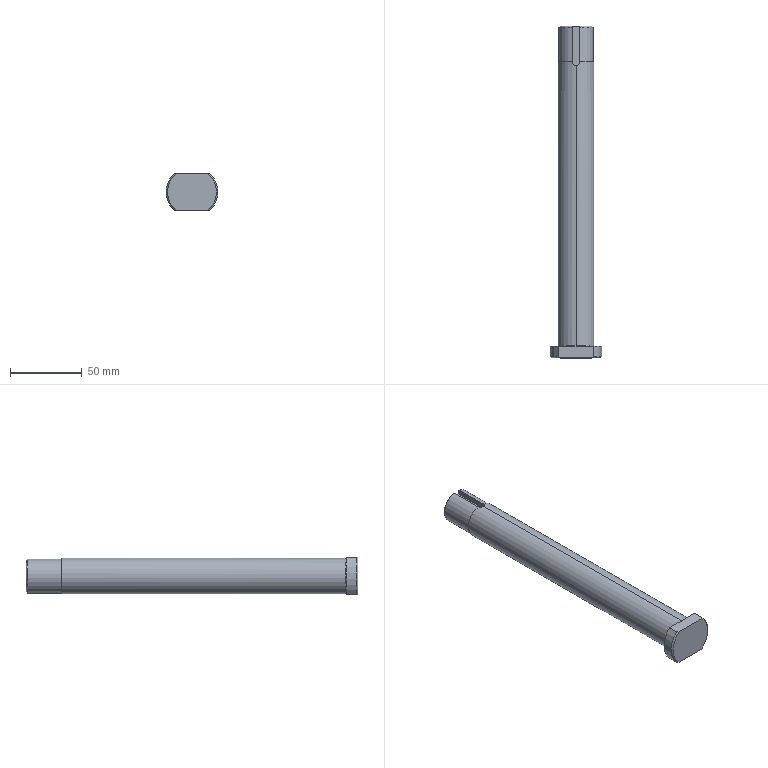Part | SolidWorks | features Chamfer 2, Fillet 2, ICE 2, Revolution 1 | 1 solid | 22 faces | box 36 x 231 x 26 mm | volume 114684 mm3 | plane 10 | cylinder 6 | cone 4 | torus 2 | commonest cylinder face diameters 25 x2 36 x2 5 x1 24 x1
STEP:
#1=CARTESIAN_POINT('',(0.,8.,13.));
#2=VERTEX_POINT('',#1);
#3=CARTESIAN_POINT('',(0.,8.,-13.));
#4=VERTEX_POINT('',#3);
#5=CARTESIAN_POINT('',(0.,8.,0.));
#6=DIRECTION('',(0.,-1.,0.));
#7=DIRECTION('',(0.,0.,-1.));
#8=AXIS2_PLACEMENT_3D('',#5,#6,#7);
#9=CIRCLE('',#8,13.);
#10=EDGE_CURVE('',#2,#4,#9,.T.);
#11=ORIENTED_EDGE('',*,*,#10,.F.);
#12=CARTESIAN_POINT('',(0.,8.5,12.5));
#13=VERTEX_POINT('',#12);
#14=CARTESIAN_POINT('',(0.,8.5,13.));
#15=DIRECTION('',(1.,0.,0.));
#16=DIRECTION('',(0.,0.,-1.));
#17=AXIS2_PLACEMENT_3D('',#14,#15,#16);
#18=CIRCLE('',#17,0.5);
#19=EDGE_CURVE('',#2,#13,#18,.T.);
#20=ORIENTED_EDGE('',*,*,#19,.T.);
#21=CARTESIAN_POINT('',(0.,8.5,-12.5));
#22=VERTEX_POINT('',#21);
#23=CARTESIAN_POINT('',(0.,8.5,0.));
#24=DIRECTION('',(0.,1.,0.));
#25=DIRECTION('',(0.,0.,-1.));
#26=AXIS2_PLACEMENT_3D('',#23,#24,#25);
#27=CIRCLE('',#26,12.5);
#28=EDGE_CURVE('',#22,#13,#27,.T.);
#29=ORIENTED_EDGE('',*,*,#28,.F.);
#30=CARTESIAN_POINT('',(0.,8.5,-13.));
#31=DIRECTION('',(-1.,0.,0.));
#32=DIRECTION('',(0.,0.,1.));
#33=AXIS2_PLACEMENT_3D('',#30,#31,#32);
#34=CIRCLE('',#33,0.5);
#35=EDGE_CURVE('',#4,#22,#34,.T.);
#36=ORIENTED_EDGE('',*,*,#35,.F.);
#37=EDGE_LOOP('',(#11,#20,#29,#36));
#38=FACE_OUTER_BOUND('',#37,.T.);
#39=CARTESIAN_POINT('',(0.,8.5,0.));
#40=DIRECTION('',(0.,-1.,0.));
#41=DIRECTION('',(0.,0.,-1.));
#42=AXIS2_PLACEMENT_3D('',#39,#40,#41);
#43=TOROIDAL_SURFACE('',#42,13.,0.5);
#44=ADVANCED_FACE('',(#38),#43,.F.);
#45=CARTESIAN_POINT('',(0.,231.,-11.));
#46=VERTEX_POINT('',#45);
#47=CARTESIAN_POINT('',(-2.5,231.,10.712));
#48=VERTEX_POINT('',#47);
#49=CARTESIAN_POINT('',(0.,231.,0.));
#50=DIRECTION('',(0.,1.,0.));
#51=DIRECTION('',(0.,0.,-1.));
#52=AXIS2_PLACEMENT_3D('',#49,#50,#51);
#53=CIRCLE('',#52,11.);
#54=EDGE_CURVE('',#46,#48,#53,.T.);
#55=ORIENTED_EDGE('',*,*,#54,.F.);
#56=CARTESIAN_POINT('',(0.,230.,-12.));
#57=VERTEX_POINT('',#56);
#58=CARTESIAN_POINT('',(0.,231.,-11.));
#59=DIRECTION('',(0.,-0.7071,-0.7071));
#60=VECTOR('',#59,1000.);
#61=LINE('',#58,#60);
#62=EDGE_CURVE('',#46,#57,#61,.T.);
#63=ORIENTED_EDGE('',*,*,#62,.T.);
#64=CARTESIAN_POINT('',(-2.5,230.,11.737));
#65=VERTEX_POINT('',#64);
#66=CARTESIAN_POINT('',(0.,230.,0.));
#67=DIRECTION('',(0.,-1.,0.));
#68=DIRECTION('',(0.,0.,-1.));
#69=AXIS2_PLACEMENT_3D('',#66,#67,#68);
#70=CIRCLE('',#69,12.);
#71=EDGE_CURVE('',#65,#57,#70,.T.);
#72=ORIENTED_EDGE('',*,*,#71,.F.);
#73=CARTESIAN_POINT('',(-2.5,231.,10.712));
#74=CARTESIAN_POINT('',(-2.5,230.667,11.054));
#75=CARTESIAN_POINT('',(-2.5,230.334,11.396));
#76=CARTESIAN_POINT('',(-2.5,230.,11.737));
#77=B_SPLINE_CURVE_WITH_KNOTS('',3,(#73,#74,#75,#76),.UNSPECIFIED.,.F.,.F.,(4,4),(0.,0.001432),.UNSPECIFIED.);
#78=EDGE_CURVE('',#48,#65,#77,.T.);
#79=ORIENTED_EDGE('',*,*,#78,.F.);
#80=EDGE_LOOP('',(#55,#63,#72,#79));
#81=FACE_OUTER_BOUND('',#80,.T.);
#82=CARTESIAN_POINT('',(0.,231.,0.));
#83=DIRECTION('',(0.,-1.,0.));
#84=DIRECTION('',(0.,0.,-1.));
#85=AXIS2_PLACEMENT_3D('',#82,#83,#84);
#86=CONICAL_SURFACE('',#85,11.,0.7854);
#87=ADVANCED_FACE('',(#81),#86,.T.);
#88=CARTESIAN_POINT('',(0.,8.5,0.));
#89=DIRECTION('',(0.,1.,0.));
#90=DIRECTION('',(0.,0.,-1.));
#91=AXIS2_PLACEMENT_3D('',#88,#89,#90);
#92=CIRCLE('',#91,12.5);
#93=EDGE_CURVE('',#13,#22,#92,.T.);
#94=ORIENTED_EDGE('',*,*,#93,.T.);
#95=CARTESIAN_POINT('',(0.,206.,-12.5));
#96=VERTEX_POINT('',#95);
#97=CARTESIAN_POINT('',(0.,0.,-12.5));
#98=DIRECTION('',(0.,1.,0.));
#99=VECTOR('',#98,1000.);
#100=LINE('',#97,#99);
#101=EDGE_CURVE('',#22,#96,#100,.T.);
#102=ORIENTED_EDGE('',*,*,#101,.T.);
#103=CARTESIAN_POINT('',(2.5,206.,12.247));
#104=VERTEX_POINT('',#103);
#105=CARTESIAN_POINT('',(0.,206.,0.));
#106=DIRECTION('',(0.,1.,0.));
#107=DIRECTION('',(0.,0.,1.));
#108=AXIS2_PLACEMENT_3D('',#105,#106,#107);
#109=CIRCLE('',#108,12.5);
#110=EDGE_CURVE('',#104,#96,#109,.T.);
#111=ORIENTED_EDGE('',*,*,#110,.F.);
#112=CARTESIAN_POINT('',(0.,203.5,12.5));
#113=VERTEX_POINT('',#112);
#114=CARTESIAN_POINT('',(2.5,206.,12.247));
#115=CARTESIAN_POINT('',(2.5,205.834,12.247));
#116=CARTESIAN_POINT('',(2.484,205.672,12.251));
#117=CARTESIAN_POINT('',(2.42,205.351,12.264));
#118=CARTESIAN_POINT('',(2.372,205.192,12.273));
#119=CARTESIAN_POINT('',(2.246,204.89,12.297));
#120=CARTESIAN_POINT('',(2.169,204.746,12.311));
#121=CARTESIAN_POINT('',(1.987,204.475,12.341));
#122=CARTESIAN_POINT('',(1.882,204.346,12.358));
#123=CARTESIAN_POINT('',(1.537,204.002,12.407));
#124=CARTESIAN_POINT('',(1.258,203.815,12.44));
#125=CARTESIAN_POINT('',(0.8073,203.628,12.475));
#126=CARTESIAN_POINT('',(0.6491,203.58,12.484));
#127=CARTESIAN_POINT('',(0.3261,203.516,12.497));
#128=CARTESIAN_POINT('',(0.1636,203.5,12.5));
#129=CARTESIAN_POINT('',(0.,203.5,12.5));
#130=B_SPLINE_CURVE_WITH_KNOTS('',3,(#114,#115,#116,#117,#118,#119,#120,#121,#122,#123,#124,#125,#126,#127,#128,#129),.UNSPECIFIED.,.F.,.F.,(4,2,2,2,2,2,2,4),(0.,0.0004899,0.0009797,0.00147,0.001959,0.002939,0.003429,0.003919),.UNSPECIFIED.);
#131=EDGE_CURVE('',#104,#113,#130,.T.);
#132=ORIENTED_EDGE('',*,*,#131,.T.);
#133=CARTESIAN_POINT('',(0.,0.,12.5));
#134=DIRECTION('',(0.,1.,0.));
#135=VECTOR('',#134,1000.);
#136=LINE('',#133,#135);
#137=EDGE_CURVE('',#13,#113,#136,.T.);
#138=ORIENTED_EDGE('',*,*,#137,.F.);
#139=EDGE_LOOP('',(#94,#102,#111,#132,#138));
#140=FACE_OUTER_BOUND('',#139,.T.);
#141=CARTESIAN_POINT('',(0.,0.,0.));
#142=DIRECTION('',(0.,1.,0.));
#143=DIRECTION('',(0.,0.,1.));
#144=AXIS2_PLACEMENT_3D('',#141,#142,#143);
#145=CYLINDRICAL_SURFACE('',#144,12.5);
#146=ADVANCED_FACE('',(#140),#145,.T.);
#147=CARTESIAN_POINT('',(-12.45,8.,13.));
#148=VERTEX_POINT('',#147);
#149=CARTESIAN_POINT('',(18.,8.,13.));
#150=DIRECTION('',(1.,0.,0.));
#151=VECTOR('',#150,1000.);
#152=LINE('',#149,#151);
#153=EDGE_CURVE('',#148,#2,#152,.T.);
#154=ORIENTED_EDGE('',*,*,#153,.T.);
#155=ORIENTED_EDGE('',*,*,#10,.T.);
#156=CARTESIAN_POINT('',(-12.45,8.,-13.));
#157=VERTEX_POINT('',#156);
#158=CARTESIAN_POINT('',(18.,8.,-13.));
#159=DIRECTION('',(-1.,0.,0.));
#160=VECTOR('',#159,1000.);
#161=LINE('',#158,#160);
#162=EDGE_CURVE('',#4,#157,#161,.T.);
#163=ORIENTED_EDGE('',*,*,#162,.T.);
#164=CARTESIAN_POINT('',(0.,8.,0.));
#165=DIRECTION('',(0.,1.,0.));
#166=DIRECTION('',(0.,0.,1.));
#167=AXIS2_PLACEMENT_3D('',#164,#165,#166);
#168=CIRCLE('',#167,18.);
#169=EDGE_CURVE('',#157,#148,#168,.T.);
#170=ORIENTED_EDGE('',*,*,#169,.T.);
#171=EDGE_LOOP('',(#154,#155,#163,#170));
#172=FACE_OUTER_BOUND('',#171,.T.);
#173=CARTESIAN_POINT('',(18.,8.,0.));
#174=DIRECTION('',(0.,-1.,0.));
#175=DIRECTION('',(0.,0.,-1.));
#176=AXIS2_PLACEMENT_3D('',#173,#174,#175);
#177=PLANE('',#176);
#178=ADVANCED_FACE('',(#172),#177,.F.);
#179=ORIENTED_EDGE('',*,*,#101,.F.);
#180=ORIENTED_EDGE('',*,*,#28,.T.);
#181=ORIENTED_EDGE('',*,*,#137,.T.);
#182=CARTESIAN_POINT('',(-2.5,206.,12.247));
#183=VERTEX_POINT('',#182);
#184=CARTESIAN_POINT('',(0.,203.5,12.5));
#185=CARTESIAN_POINT('',(-0.1634,203.5,12.5));
#186=CARTESIAN_POINT('',(-0.3294,203.516,12.497));
#187=CARTESIAN_POINT('',(-0.6501,203.58,12.484));
#188=CARTESIAN_POINT('',(-0.806,203.628,12.475));
#189=CARTESIAN_POINT('',(-1.109,203.753,12.452));
#190=CARTESIAN_POINT('',(-1.255,203.832,12.438));
#191=CARTESIAN_POINT('',(-1.525,204.012,12.407));
#192=CARTESIAN_POINT('',(-1.651,204.116,12.391));
#193=CARTESIAN_POINT('',(-1.884,204.348,12.358));
#194=CARTESIAN_POINT('',(-1.987,204.474,12.341));
#195=CARTESIAN_POINT('',(-2.168,204.744,12.311));
#196=CARTESIAN_POINT('',(-2.246,204.89,12.297));
#197=CARTESIAN_POINT('',(-2.371,205.192,12.273));
#198=CARTESIAN_POINT('',(-2.419,205.348,12.264));
#199=CARTESIAN_POINT('',(-2.483,205.669,12.251));
#200=CARTESIAN_POINT('',(-2.5,205.834,12.247));
#201=CARTESIAN_POINT('',(-2.5,206.,12.247));
#202=B_SPLINE_CURVE_WITH_KNOTS('',3,(#184,#185,#186,#187,#188,#189,#190,#191,#192,#193,#194,#195,#196,#197,#198,#199,#200,#201),.UNSPECIFIED.,.F.,.F.,(4,2,2,2,2,2,2,2,4),(0.003919,0.004408,0.004898,0.005387,0.005876,0.006366,0.006855,0.007344,0.007834),.UNSPECIFIED.);
#203=EDGE_CURVE('',#113,#183,#202,.T.);
#204=ORIENTED_EDGE('',*,*,#203,.T.);
#205=CARTESIAN_POINT('',(0.,206.,0.));
#206=DIRECTION('',(0.,1.,0.));
#207=DIRECTION('',(0.,0.,1.));
#208=AXIS2_PLACEMENT_3D('',#205,#206,#207);
#209=CIRCLE('',#208,12.5);
#210=EDGE_CURVE('',#96,#183,#209,.T.);
#211=ORIENTED_EDGE('',*,*,#210,.F.);
#212=EDGE_LOOP('',(#179,#180,#181,#204,#211));
#213=FACE_OUTER_BOUND('',#212,.T.);
#214=CARTESIAN_POINT('',(0.,0.,0.));
#215=DIRECTION('',(0.,1.,0.));
#216=DIRECTION('',(0.,0.,1.));
#217=AXIS2_PLACEMENT_3D('',#214,#215,#216);
#218=CYLINDRICAL_SURFACE('',#217,12.5);
#219=ADVANCED_FACE('',(#213),#218,.T.);
#220=CARTESIAN_POINT('',(-2.5,206.,11.737));
#221=VERTEX_POINT('',#220);
#222=CARTESIAN_POINT('',(-2.5,206.,13.001));
#223=DIRECTION('',(0.,0.,-1.));
#224=VECTOR('',#223,1000.);
#225=LINE('',#222,#224);
#226=EDGE_CURVE('',#183,#221,#225,.T.);
#227=ORIENTED_EDGE('',*,*,#226,.T.);
#228=CARTESIAN_POINT('',(2.5,206.,11.737));
#229=VERTEX_POINT('',#228);
#230=CARTESIAN_POINT('',(0.,206.,0.));
#231=DIRECTION('',(0.,1.,0.));
#232=DIRECTION('',(0.,0.,1.));
#233=AXIS2_PLACEMENT_3D('',#230,#231,#232);
#234=CIRCLE('',#233,12.);
#235=EDGE_CURVE('',#229,#221,#234,.T.);
#236=ORIENTED_EDGE('',*,*,#235,.F.);
#237=CARTESIAN_POINT('',(2.5,206.,13.001));
#238=DIRECTION('',(0.,0.,-1.));
#239=VECTOR('',#238,1000.);
#240=LINE('',#237,#239);
#241=EDGE_CURVE('',#104,#229,#240,.T.);
#242=ORIENTED_EDGE('',*,*,#241,.F.);
#243=ORIENTED_EDGE('',*,*,#110,.T.);
#244=ORIENTED_EDGE('',*,*,#210,.T.);
#245=EDGE_LOOP('',(#227,#236,#242,#243,#244));
#246=FACE_OUTER_BOUND('',#245,.T.);
#247=CARTESIAN_POINT('',(12.5,206.,0.));
#248=DIRECTION('',(0.,-1.,0.));
#249=DIRECTION('',(0.,0.,-1.));
#250=AXIS2_PLACEMENT_3D('',#247,#248,#249);
#251=PLANE('',#250);
#252=ADVANCED_FACE('',(#246),#251,.F.);
#253=CARTESIAN_POINT('',(-2.5,0.,11.737));
#254=DIRECTION('',(0.,1.,0.));
#255=VECTOR('',#254,1000.);
#256=LINE('',#253,#255);
#257=EDGE_CURVE('',#221,#65,#256,.T.);
#258=ORIENTED_EDGE('',*,*,#257,.T.);
#259=ORIENTED_EDGE('',*,*,#71,.T.);
#260=CARTESIAN_POINT('',(2.5,230.,11.737));
#261=VERTEX_POINT('',#260);
#262=CARTESIAN_POINT('',(0.,230.,0.));
#263=DIRECTION('',(0.,-1.,0.));
#264=DIRECTION('',(0.,0.,-1.));
#265=AXIS2_PLACEMENT_3D('',#262,#263,#264);
#266=CIRCLE('',#265,12.);
#267=EDGE_CURVE('',#57,#261,#266,.T.);
#268=ORIENTED_EDGE('',*,*,#267,.T.);
#269=CARTESIAN_POINT('',(2.5,0.,11.737));
#270=DIRECTION('',(0.,-1.,0.));
#271=VECTOR('',#270,1000.);
#272=LINE('',#269,#271);
#273=EDGE_CURVE('',#261,#229,#272,.T.);
#274=ORIENTED_EDGE('',*,*,#273,.T.);
#275=ORIENTED_EDGE('',*,*,#235,.T.);
#276=EDGE_LOOP('',(#258,#259,#268,#274,#275));
#277=FACE_OUTER_BOUND('',#276,.T.);
#278=CARTESIAN_POINT('',(0.,0.,0.));
#279=DIRECTION('',(0.,1.,0.));
#280=DIRECTION('',(0.,0.,1.));
#281=AXIS2_PLACEMENT_3D('',#278,#279,#280);
#282=CYLINDRICAL_SURFACE('',#281,12.);
#283=ADVANCED_FACE('',(#277),#282,.T.);
#284=CARTESIAN_POINT('',(2.5,231.,8.));
#285=VERTEX_POINT('',#284);
#286=CARTESIAN_POINT('',(2.5,231.,10.712));
#287=VERTEX_POINT('',#286);
#288=CARTESIAN_POINT('',(2.5,231.,13.001));
#289=DIRECTION('',(0.,0.,1.));
#290=VECTOR('',#289,1000.);
#291=LINE('',#288,#290);
#292=EDGE_CURVE('',#285,#287,#291,.T.);
#293=ORIENTED_EDGE('',*,*,#292,.T.);
#294=CARTESIAN_POINT('',(0.,231.,0.));
#295=DIRECTION('',(0.,1.,0.));
#296=DIRECTION('',(0.,0.,-1.));
#297=AXIS2_PLACEMENT_3D('',#294,#295,#296);
#298=CIRCLE('',#297,11.);
#299=EDGE_CURVE('',#287,#46,#298,.T.);
#300=ORIENTED_EDGE('',*,*,#299,.T.);
#301=ORIENTED_EDGE('',*,*,#54,.T.);
#302=CARTESIAN_POINT('',(-2.5,231.,8.));
#303=VERTEX_POINT('',#302);
#304=CARTESIAN_POINT('',(-2.5,231.,13.001));
#305=DIRECTION('',(0.,0.,-1.));
#306=VECTOR('',#305,1000.);
#307=LINE('',#304,#306);
#308=EDGE_CURVE('',#48,#303,#307,.T.);
#309=ORIENTED_EDGE('',*,*,#308,.T.);
#310=CARTESIAN_POINT('',(0.,231.,8.));
#311=DIRECTION('',(1.,0.,0.));
#312=VECTOR('',#311,1000.);
#313=LINE('',#310,#312);
#314=EDGE_CURVE('',#303,#285,#313,.T.);
#315=ORIENTED_EDGE('',*,*,#314,.T.);
#316=EDGE_LOOP('',(#293,#300,#301,#309,#315));
#317=FACE_OUTER_BOUND('',#316,.T.);
#318=CARTESIAN_POINT('',(12.,231.,0.));
#319=DIRECTION('',(0.,-1.,0.));
#320=DIRECTION('',(0.,0.,-1.));
#321=AXIS2_PLACEMENT_3D('',#318,#319,#320);
#322=PLANE('',#321);
#323=ADVANCED_FACE('',(#317),#322,.F.);
#324=CARTESIAN_POINT('',(-12.45,1.,-13.));
#325=VERTEX_POINT('',#324);
#326=CARTESIAN_POINT('',(-12.45,0.,-13.));
#327=DIRECTION('',(0.,-1.,0.));
#328=VECTOR('',#327,1000.);
#329=LINE('',#326,#328);
#330=EDGE_CURVE('',#157,#325,#329,.T.);
#331=ORIENTED_EDGE('',*,*,#330,.T.);
#332=CARTESIAN_POINT('',(-12.45,1.,13.));
#333=VERTEX_POINT('',#332);
#334=CARTESIAN_POINT('',(0.,1.,0.));
#335=DIRECTION('',(0.,1.,0.));
#336=DIRECTION('',(0.,0.,1.));
#337=AXIS2_PLACEMENT_3D('',#334,#335,#336);
#338=CIRCLE('',#337,18.);
#339=EDGE_CURVE('',#325,#333,#338,.T.);
#340=ORIENTED_EDGE('',*,*,#339,.T.);
#341=CARTESIAN_POINT('',(-12.45,0.,13.));
#342=DIRECTION('',(0.,1.,0.));
#343=VECTOR('',#342,1000.);
#344=LINE('',#341,#343);
#345=EDGE_CURVE('',#333,#148,#344,.T.);
#346=ORIENTED_EDGE('',*,*,#345,.T.);
#347=ORIENTED_EDGE('',*,*,#169,.F.);
#348=EDGE_LOOP('',(#331,#340,#346,#347));
#349=FACE_OUTER_BOUND('',#348,.T.);
#350=CARTESIAN_POINT('',(0.,0.,0.));
#351=DIRECTION('',(0.,1.,0.));
#352=DIRECTION('',(0.,0.,1.));
#353=AXIS2_PLACEMENT_3D('',#350,#351,#352);
#354=CYLINDRICAL_SURFACE('',#353,18.);
#355=ADVANCED_FACE('',(#349),#354,.T.);
#356=CARTESIAN_POINT('',(-10.954,0.,13.));
#357=VERTEX_POINT('',#356);
#358=CARTESIAN_POINT('',(10.954,0.,13.));
#359=VERTEX_POINT('',#358);
#360=CARTESIAN_POINT('',(65.,0.,13.));
#361=DIRECTION('',(1.,0.,0.));
#362=VECTOR('',#361,1000.);
#363=LINE('',#360,#362);
#364=EDGE_CURVE('',#357,#359,#363,.T.);
#365=ORIENTED_EDGE('',*,*,#364,.F.);
#366=CARTESIAN_POINT('',(-10.954,0.,-13.));
#367=VERTEX_POINT('',#366);
#368=CARTESIAN_POINT('',(0.,0.,0.));
#369=DIRECTION('',(0.,-1.,0.));
#370=DIRECTION('',(0.,0.,1.));
#371=AXIS2_PLACEMENT_3D('',#368,#369,#370);
#372=CIRCLE('',#371,17.);
#373=EDGE_CURVE('',#357,#367,#372,.T.);
#374=ORIENTED_EDGE('',*,*,#373,.T.);
#375=CARTESIAN_POINT('',(10.954,0.,-13.));
#376=VERTEX_POINT('',#375);
#377=CARTESIAN_POINT('',(65.,0.,-13.));
#378=DIRECTION('',(-1.,0.,0.));
#379=VECTOR('',#378,1000.);
#380=LINE('',#377,#379);
#381=EDGE_CURVE('',#376,#367,#380,.T.);
#382=ORIENTED_EDGE('',*,*,#381,.F.);
#383=CARTESIAN_POINT('',(0.,0.,0.));
#384=DIRECTION('',(0.,-1.,0.));
#385=DIRECTION('',(0.,0.,1.));
#386=AXIS2_PLACEMENT_3D('',#383,#384,#385);
#387=CIRCLE('',#386,17.);
#388=EDGE_CURVE('',#376,#359,#387,.T.);
#389=ORIENTED_EDGE('',*,*,#388,.T.);
#390=EDGE_LOOP('',(#365,#374,#382,#389));
#391=FACE_OUTER_BOUND('',#390,.T.);
#392=CARTESIAN_POINT('',(0.,0.,0.));
#393=DIRECTION('',(0.,1.,0.));
#394=DIRECTION('',(0.,0.,1.));
#395=AXIS2_PLACEMENT_3D('',#392,#393,#394);
#396=PLANE('',#395);
#397=ADVANCED_FACE('',(#391),#396,.F.);
#398=CARTESIAN_POINT('',(12.45,8.,13.));
#399=VERTEX_POINT('',#398);
#400=CARTESIAN_POINT('',(12.45,1.,13.));
#401=VERTEX_POINT('',#400);
#402=CARTESIAN_POINT('',(12.45,0.,13.));
#403=DIRECTION('',(0.,-1.,0.));
#404=VECTOR('',#403,1000.);
#405=LINE('',#402,#404);
#406=EDGE_CURVE('',#399,#401,#405,.T.);
#407=ORIENTED_EDGE('',*,*,#406,.T.);
#408=CARTESIAN_POINT('',(12.45,1.,-13.));
#409=VERTEX_POINT('',#408);
#410=CARTESIAN_POINT('',(0.,1.,0.));
#411=DIRECTION('',(0.,1.,0.));
#412=DIRECTION('',(0.,0.,1.));
#413=AXIS2_PLACEMENT_3D('',#410,#411,#412);
#414=CIRCLE('',#413,18.);
#415=EDGE_CURVE('',#401,#409,#414,.T.);
#416=ORIENTED_EDGE('',*,*,#415,.T.);
#417=CARTESIAN_POINT('',(12.45,8.,-13.));
#418=VERTEX_POINT('',#417);
#419=CARTESIAN_POINT('',(12.45,0.,-13.));
#420=DIRECTION('',(0.,1.,0.));
#421=VECTOR('',#420,1000.);
#422=LINE('',#419,#421);
#423=EDGE_CURVE('',#409,#418,#422,.T.);
#424=ORIENTED_EDGE('',*,*,#423,.T.);
#425=CARTESIAN_POINT('',(0.,8.,0.));
#426=DIRECTION('',(0.,1.,0.));
#427=DIRECTION('',(0.,0.,1.));
#428=AXIS2_PLACEMENT_3D('',#425,#426,#427);
#429=CIRCLE('',#428,18.);
#430=EDGE_CURVE('',#399,#418,#429,.T.);
#431=ORIENTED_EDGE('',*,*,#430,.F.);
#432=EDGE_LOOP('',(#407,#416,#424,#431));
#433=FACE_OUTER_BOUND('',#432,.T.);
#434=CARTESIAN_POINT('',(0.,0.,0.));
#435=DIRECTION('',(0.,1.,0.));
#436=DIRECTION('',(0.,0.,1.));
#437=AXIS2_PLACEMENT_3D('',#434,#435,#436);
#438=CYLINDRICAL_SURFACE('',#437,18.);
#439=ADVANCED_FACE('',(#433),#438,.T.);
#440=CARTESIAN_POINT('',(18.,8.,-13.));
#441=DIRECTION('',(-1.,0.,0.));
#442=VECTOR('',#441,1000.);
#443=LINE('',#440,#442);
#444=EDGE_CURVE('',#418,#4,#443,.T.);
#445=ORIENTED_EDGE('',*,*,#444,.T.);
#446=CARTESIAN_POINT('',(0.,8.,0.));
#447=DIRECTION('',(0.,-1.,0.));
#448=DIRECTION('',(0.,0.,-1.));
#449=AXIS2_PLACEMENT_3D('',#446,#447,#448);
#450=CIRCLE('',#449,13.);
#451=EDGE_CURVE('',#4,#2,#450,.T.);
#452=ORIENTED_EDGE('',*,*,#451,.T.);
#453=CARTESIAN_POINT('',(18.,8.,13.));
#454=DIRECTION('',(1.,0.,0.));
#455=VECTOR('',#454,1000.);
#456=LINE('',#453,#455);
#457=EDGE_CURVE('',#2,#399,#456,.T.);
#458=ORIENTED_EDGE('',*,*,#457,.T.);
#459=ORIENTED_EDGE('',*,*,#430,.T.);
#460=EDGE_LOOP('',(#445,#452,#458,#459));
#461=FACE_OUTER_BOUND('',#460,.T.);
#462=CARTESIAN_POINT('',(18.,8.,0.));
#463=DIRECTION('',(0.,-1.,0.));
#464=DIRECTION('',(0.,0.,-1.));
#465=AXIS2_PLACEMENT_3D('',#462,#463,#464);
#466=PLANE('',#465);
#467=ADVANCED_FACE('',(#461),#466,.F.);
#468=ORIENTED_EDGE('',*,*,#381,.T.);
#469=CARTESIAN_POINT('',(-10.954,0.,-13.));
#470=CARTESIAN_POINT('',(-11.459,0.3249,-13.));
#471=CARTESIAN_POINT('',(-11.957,0.6588,-13.));
#472=CARTESIAN_POINT('',(-12.45,1.,-13.));
#473=B_SPLINE_CURVE_WITH_KNOTS('',3,(#469,#470,#471,#472),.UNSPECIFIED.,.F.,.F.,(4,4),(0.,0.001799),.UNSPECIFIED.);
#474=EDGE_CURVE('',#367,#325,#473,.T.);
#475=ORIENTED_EDGE('',*,*,#474,.T.);
#476=ORIENTED_EDGE('',*,*,#330,.F.);
#477=ORIENTED_EDGE('',*,*,#162,.F.);
#478=ORIENTED_EDGE('',*,*,#444,.F.);
#479=ORIENTED_EDGE('',*,*,#423,.F.);
#480=CARTESIAN_POINT('',(12.45,1.,-13.));
#481=CARTESIAN_POINT('',(11.957,0.6588,-13.));
#482=CARTESIAN_POINT('',(11.459,0.3249,-13.));
#483=CARTESIAN_POINT('',(10.954,0.,-13.));
#484=B_SPLINE_CURVE_WITH_KNOTS('',3,(#480,#481,#482,#483),.UNSPECIFIED.,.F.,.F.,(4,4),(0.,0.001799),.UNSPECIFIED.);
#485=EDGE_CURVE('',#409,#376,#484,.T.);
#486=ORIENTED_EDGE('',*,*,#485,.T.);
#487=EDGE_LOOP('',(#468,#475,#476,#477,#478,#479,#486));
#488=FACE_OUTER_BOUND('',#487,.T.);
#489=CARTESIAN_POINT('',(65.,10.,-13.));
#490=DIRECTION('',(0.,0.,1.));
#491=DIRECTION('',(1.,0.,0.));
#492=AXIS2_PLACEMENT_3D('',#489,#490,#491);
#493=PLANE('',#492);
#494=ADVANCED_FACE('',(#488),#493,.F.);
#495=ORIENTED_EDGE('',*,*,#345,.F.);
#496=CARTESIAN_POINT('',(-12.45,1.,13.));
#497=CARTESIAN_POINT('',(-11.957,0.6588,13.));
#498=CARTESIAN_POINT('',(-11.459,0.3249,13.));
#499=CARTESIAN_POINT('',(-10.954,0.,13.));
#500=B_SPLINE_CURVE_WITH_KNOTS('',3,(#496,#497,#498,#499),.UNSPECIFIED.,.F.,.F.,(4,4),(0.,0.001799),.UNSPECIFIED.);
#501=EDGE_CURVE('',#333,#357,#500,.T.);
#502=ORIENTED_EDGE('',*,*,#501,.T.);
#503=ORIENTED_EDGE('',*,*,#364,.T.);
#504=CARTESIAN_POINT('',(10.954,0.,13.));
#505=CARTESIAN_POINT('',(11.459,0.3249,13.));
#506=CARTESIAN_POINT('',(11.957,0.6588,13.));
#507=CARTESIAN_POINT('',(12.45,1.,13.));
#508=B_SPLINE_CURVE_WITH_KNOTS('',3,(#504,#505,#506,#507),.UNSPECIFIED.,.F.,.F.,(4,4),(0.,0.001799),.UNSPECIFIED.);
#509=EDGE_CURVE('',#359,#401,#508,.T.);
#510=ORIENTED_EDGE('',*,*,#509,.T.);
#511=ORIENTED_EDGE('',*,*,#406,.F.);
#512=ORIENTED_EDGE('',*,*,#457,.F.);
#513=ORIENTED_EDGE('',*,*,#153,.F.);
#514=EDGE_LOOP('',(#495,#502,#503,#510,#511,#512,#513));
#515=FACE_OUTER_BOUND('',#514,.T.);
#516=CARTESIAN_POINT('',(65.,10.,13.));
#517=DIRECTION('',(0.,0.,-1.));
#518=DIRECTION('',(-1.,0.,0.));
#519=AXIS2_PLACEMENT_3D('',#516,#517,#518);
#520=PLANE('',#519);
#521=ADVANCED_FACE('',(#515),#520,.F.);
#522=ORIENTED_EDGE('',*,*,#308,.F.);
#523=ORIENTED_EDGE('',*,*,#78,.T.);
#524=ORIENTED_EDGE('',*,*,#257,.F.);
#525=CARTESIAN_POINT('',(-2.5,206.,8.));
#526=VERTEX_POINT('',#525);
#527=CARTESIAN_POINT('',(-2.5,206.,13.001));
#528=DIRECTION('',(0.,0.,-1.));
#529=VECTOR('',#528,1000.);
#530=LINE('',#527,#529);
#531=EDGE_CURVE('',#221,#526,#530,.T.);
#532=ORIENTED_EDGE('',*,*,#531,.T.);
#533=CARTESIAN_POINT('',(-2.5,231.,8.));
#534=DIRECTION('',(0.,-1.,0.));
#535=VECTOR('',#534,1000.);
#536=LINE('',#533,#535);
#537=EDGE_CURVE('',#303,#526,#536,.T.);
#538=ORIENTED_EDGE('',*,*,#537,.F.);
#539=EDGE_LOOP('',(#522,#523,#524,#532,#538));
#540=FACE_OUTER_BOUND('',#539,.T.);
#541=CARTESIAN_POINT('',(-2.5,231.,13.001));
#542=DIRECTION('',(1.,0.,0.));
#543=DIRECTION('',(0.,1.,0.));
#544=AXIS2_PLACEMENT_3D('',#541,#542,#543);
#545=PLANE('',#544);
#546=ADVANCED_FACE('',(#540),#545,.T.);
#547=ORIENTED_EDGE('',*,*,#241,.T.);
#548=CARTESIAN_POINT('',(2.5,206.,8.));
#549=VERTEX_POINT('',#548);
#550=CARTESIAN_POINT('',(2.5,206.,13.001));
#551=DIRECTION('',(0.,0.,-1.));
#552=VECTOR('',#551,1000.);
#553=LINE('',#550,#552);
#554=EDGE_CURVE('',#229,#549,#553,.T.);
#555=ORIENTED_EDGE('',*,*,#554,.T.);
#556=CARTESIAN_POINT('',(0.,206.,8.));
#557=DIRECTION('',(0.,0.,1.));
#558=DIRECTION('',(1.,0.,0.));
#559=AXIS2_PLACEMENT_3D('',#556,#557,#558);
#560=CIRCLE('',#559,2.5);
#561=EDGE_CURVE('',#526,#549,#560,.T.);
#562=ORIENTED_EDGE('',*,*,#561,.F.);
#563=ORIENTED_EDGE('',*,*,#531,.F.);
#564=ORIENTED_EDGE('',*,*,#226,.F.);
#565=ORIENTED_EDGE('',*,*,#203,.F.);
#566=ORIENTED_EDGE('',*,*,#131,.F.);
#567=EDGE_LOOP('',(#547,#555,#562,#563,#564,#565,#566));
#568=FACE_OUTER_BOUND('',#567,.T.);
#569=CARTESIAN_POINT('',(0.,206.,13.001));
#570=DIRECTION('',(0.,0.,-1.));
#571=DIRECTION('',(-1.,0.,0.));
#572=AXIS2_PLACEMENT_3D('',#569,#570,#571);
#573=CYLINDRICAL_SURFACE('',#572,2.5);
#574=ADVANCED_FACE('',(#568),#573,.F.);
#575=ORIENTED_EDGE('',*,*,#273,.F.);
#576=CARTESIAN_POINT('',(2.5,230.,11.737));
#577=CARTESIAN_POINT('',(2.5,230.334,11.396));
#578=CARTESIAN_POINT('',(2.5,230.667,11.054));
#579=CARTESIAN_POINT('',(2.5,231.,10.712));
#580=B_SPLINE_CURVE_WITH_KNOTS('',3,(#576,#577,#578,#579),.UNSPECIFIED.,.F.,.F.,(4,4),(0.,0.001432),.UNSPECIFIED.);
#581=EDGE_CURVE('',#261,#287,#580,.T.);
#582=ORIENTED_EDGE('',*,*,#581,.T.);
#583=ORIENTED_EDGE('',*,*,#292,.F.);
#584=CARTESIAN_POINT('',(2.5,231.,8.));
#585=DIRECTION('',(0.,1.,0.));
#586=VECTOR('',#585,1000.);
#587=LINE('',#584,#586);
#588=EDGE_CURVE('',#549,#285,#587,.T.);
#589=ORIENTED_EDGE('',*,*,#588,.F.);
#590=ORIENTED_EDGE('',*,*,#554,.F.);
#591=EDGE_LOOP('',(#575,#582,#583,#589,#590));
#592=FACE_OUTER_BOUND('',#591,.T.);
#593=CARTESIAN_POINT('',(2.5,231.,13.001));
#594=DIRECTION('',(-1.,0.,0.));
#595=DIRECTION('',(0.,-1.,0.));
#596=AXIS2_PLACEMENT_3D('',#593,#594,#595);
#597=PLANE('',#596);
#598=ADVANCED_FACE('',(#592),#597,.T.);
#599=ORIENTED_EDGE('',*,*,#537,.T.);
#600=ORIENTED_EDGE('',*,*,#561,.T.);
#601=ORIENTED_EDGE('',*,*,#588,.T.);
#602=ORIENTED_EDGE('',*,*,#314,.F.);
#603=EDGE_LOOP('',(#599,#600,#601,#602));
#604=FACE_OUTER_BOUND('',#603,.T.);
#605=CARTESIAN_POINT('',(0.,231.,8.));
#606=DIRECTION('',(0.,0.,1.));
#607=DIRECTION('',(1.,0.,0.));
#608=AXIS2_PLACEMENT_3D('',#605,#606,#607);
#609=PLANE('',#608);
#610=ADVANCED_FACE('',(#604),#609,.T.);
#611=ORIENTED_EDGE('',*,*,#62,.F.);
#612=ORIENTED_EDGE('',*,*,#299,.F.);
#613=ORIENTED_EDGE('',*,*,#581,.F.);
#614=ORIENTED_EDGE('',*,*,#267,.F.);
#615=EDGE_LOOP('',(#611,#612,#613,#614));
#616=FACE_OUTER_BOUND('',#615,.T.);
#617=CARTESIAN_POINT('',(0.,231.,0.));
#618=DIRECTION('',(0.,-1.,0.));
#619=DIRECTION('',(0.,0.,-1.));
#620=AXIS2_PLACEMENT_3D('',#617,#618,#619);
#621=CONICAL_SURFACE('',#620,11.,0.7854);
#622=ADVANCED_FACE('',(#616),#621,.T.);
#623=ORIENTED_EDGE('',*,*,#19,.F.);
#624=ORIENTED_EDGE('',*,*,#451,.F.);
#625=ORIENTED_EDGE('',*,*,#35,.T.);
#626=ORIENTED_EDGE('',*,*,#93,.F.);
#627=EDGE_LOOP('',(#623,#624,#625,#626));
#628=FACE_OUTER_BOUND('',#627,.T.);
#629=CARTESIAN_POINT('',(0.,8.5,0.));
#630=DIRECTION('',(0.,-1.,0.));
#631=DIRECTION('',(0.,0.,-1.));
#632=AXIS2_PLACEMENT_3D('',#629,#630,#631);
#633=TOROIDAL_SURFACE('',#632,13.,0.5);
#634=ADVANCED_FACE('',(#628),#633,.F.);
#635=ORIENTED_EDGE('',*,*,#474,.F.);
#636=ORIENTED_EDGE('',*,*,#373,.F.);
#637=ORIENTED_EDGE('',*,*,#501,.F.);
#638=ORIENTED_EDGE('',*,*,#339,.F.);
#639=EDGE_LOOP('',(#635,#636,#637,#638));
#640=FACE_OUTER_BOUND('',#639,.T.);
#641=CARTESIAN_POINT('',(0.,1.,0.));
#642=DIRECTION('',(0.,1.,0.));
#643=DIRECTION('',(0.,0.,1.));
#644=AXIS2_PLACEMENT_3D('',#641,#642,#643);
#645=CONICAL_SURFACE('',#644,18.,0.7854);
#646=ADVANCED_FACE('',(#640),#645,.T.);
#647=ORIENTED_EDGE('',*,*,#509,.F.);
#648=ORIENTED_EDGE('',*,*,#388,.F.);
#649=ORIENTED_EDGE('',*,*,#485,.F.);
#650=ORIENTED_EDGE('',*,*,#415,.F.);
#651=EDGE_LOOP('',(#647,#648,#649,#650));
#652=FACE_OUTER_BOUND('',#651,.T.);
#653=CARTESIAN_POINT('',(0.,1.,0.));
#654=DIRECTION('',(0.,1.,0.));
#655=DIRECTION('',(0.,0.,1.));
#656=AXIS2_PLACEMENT_3D('',#653,#654,#655);
#657=CONICAL_SURFACE('',#656,18.,0.7854);
#658=ADVANCED_FACE('',(#652),#657,.T.);
#659=CLOSED_SHELL('',(#44,#87,#146,#178,#219,#252,#283,#323,#355,#397,#439,#467,#494,#521,#546,#574,#598,#610,#622,#634,#646,#658));
#660=MANIFOLD_SOLID_BREP('',#659);
#661=CARTESIAN_POINT('',(0.,0.,0.));
#662=DIRECTION('',(0.,0.,1.));
#663=DIRECTION('',(1.,0.,0.));
#664=AXIS2_PLACEMENT_3D('',#661,#662,#663);
#665=(LENGTH_UNIT()NAMED_UNIT(*)SI_UNIT(.MILLI.,.METRE.));
#666=UNCERTAINTY_MEASURE_WITH_UNIT(LENGTH_MEASURE(0.00001),#665,'','');
#667=(NAMED_UNIT(*)PLANE_ANGLE_UNIT()SI_UNIT($,.RADIAN.));
#668=(NAMED_UNIT(*)SI_UNIT($,.STERADIAN.)SOLID_ANGLE_UNIT());
#669=(GEOMETRIC_REPRESENTATION_CONTEXT(3)GLOBAL_UNCERTAINTY_ASSIGNED_CONTEXT((#666))GLOBAL_UNIT_ASSIGNED_CONTEXT((#665,#667,#668))REPRESENTATION_CONTEXT('',''));
#670=ADVANCED_BREP_SHAPE_REPRESENTATION('',(#660,#664),#669);